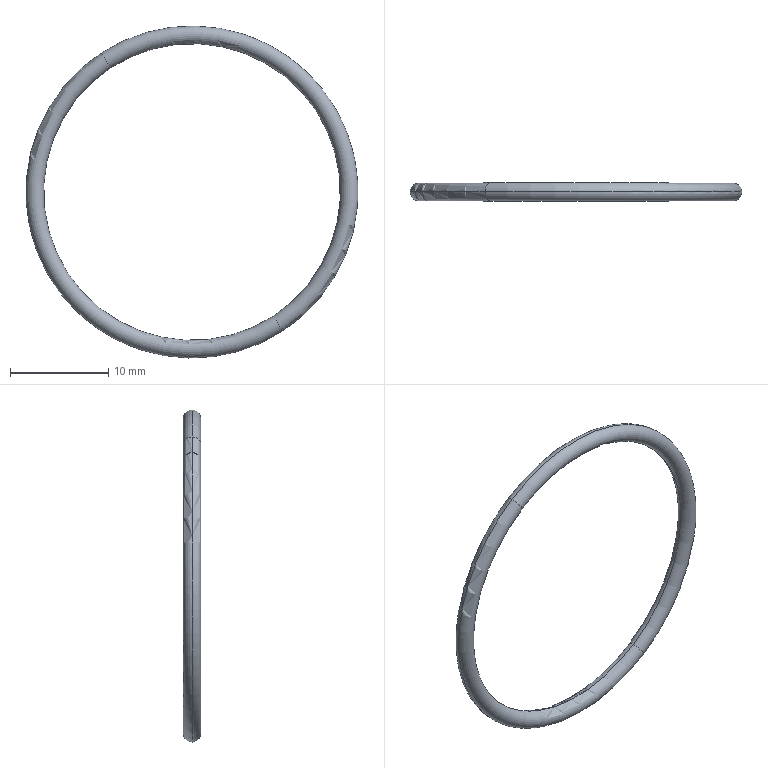Part | SolidWorks | features BaseBody 1 | 1 solid | 4 faces | box 33.8 x 1.8 x 33.8 mm | volume 255.82 mm3 | torus 4
STEP:
#1=CARTESIAN_POINT('',(218.757,-105.5,303.648));
#2=VERTEX_POINT('',#1);
#3=CARTESIAN_POINT('',(219.741,-105.5,302.141));
#4=VERTEX_POINT('',#3);
#5=CARTESIAN_POINT('',(219.249,-105.5,302.895));
#6=DIRECTION('',(-0.8372,0.,-0.5469));
#7=DIRECTION('',(-0.5469,0.,0.8372));
#8=AXIS2_PLACEMENT_3D('',#5,#6,#7);
#9=CIRCLE('',#8,0.9);
#10=EDGE_CURVE('',#2,#4,#9,.T.);
#11=ORIENTED_EDGE('',*,*,#10,.F.);
#12=CARTESIAN_POINT('',(237.243,-105.5,275.352));
#13=VERTEX_POINT('',#12);
#14=CARTESIAN_POINT('',(228.,-105.5,289.5));
#15=DIRECTION('',(0.,1.,0.));
#16=DIRECTION('',(0.,0.,1.));
#17=AXIS2_PLACEMENT_3D('',#14,#15,#16);
#18=CIRCLE('',#17,16.9);
#19=EDGE_CURVE('',#2,#13,#18,.T.);
#20=ORIENTED_EDGE('',*,*,#19,.T.);
#21=CARTESIAN_POINT('',(236.259,-105.5,276.859));
#22=VERTEX_POINT('',#21);
#23=CARTESIAN_POINT('',(236.751,-105.5,276.105));
#24=DIRECTION('',(0.8372,0.,0.5469));
#25=DIRECTION('',(0.5469,0.,-0.8372));
#26=AXIS2_PLACEMENT_3D('',#23,#24,#25);
#27=CIRCLE('',#26,0.9);
#28=EDGE_CURVE('',#13,#22,#27,.T.);
#29=ORIENTED_EDGE('',*,*,#28,.T.);
#30=CARTESIAN_POINT('',(228.,-105.5,289.5));
#31=DIRECTION('',(0.,1.,0.));
#32=DIRECTION('',(0.,0.,1.));
#33=AXIS2_PLACEMENT_3D('',#30,#31,#32);
#34=CIRCLE('',#33,15.1);
#35=EDGE_CURVE('',#4,#22,#34,.T.);
#36=ORIENTED_EDGE('',*,*,#35,.F.);
#37=EDGE_LOOP('',(#11,#20,#29,#36));
#38=FACE_OUTER_BOUND('',#37,.T.);
#39=CARTESIAN_POINT('',(228.,-105.5,289.5));
#40=DIRECTION('',(0.,1.,0.));
#41=DIRECTION('',(0.5469,0.,-0.8372));
#42=AXIS2_PLACEMENT_3D('',#39,#40,#41);
#43=TOROIDAL_SURFACE('',#42,16.,0.9);
#44=ADVANCED_FACE('',(#38),#43,.T.);
#45=ORIENTED_EDGE('',*,*,#28,.F.);
#46=CARTESIAN_POINT('',(228.,-105.5,289.5));
#47=DIRECTION('',(0.,1.,0.));
#48=DIRECTION('',(0.,0.,1.));
#49=AXIS2_PLACEMENT_3D('',#46,#47,#48);
#50=CIRCLE('',#49,16.9);
#51=EDGE_CURVE('',#13,#2,#50,.T.);
#52=ORIENTED_EDGE('',*,*,#51,.T.);
#53=ORIENTED_EDGE('',*,*,#10,.T.);
#54=CARTESIAN_POINT('',(228.,-105.5,289.5));
#55=DIRECTION('',(0.,1.,0.));
#56=DIRECTION('',(0.,0.,1.));
#57=AXIS2_PLACEMENT_3D('',#54,#55,#56);
#58=CIRCLE('',#57,15.1);
#59=EDGE_CURVE('',#22,#4,#58,.T.);
#60=ORIENTED_EDGE('',*,*,#59,.F.);
#61=EDGE_LOOP('',(#45,#52,#53,#60));
#62=FACE_OUTER_BOUND('',#61,.T.);
#63=CARTESIAN_POINT('',(228.,-105.5,289.5));
#64=DIRECTION('',(0.,1.,0.));
#65=DIRECTION('',(0.5469,0.,-0.8372));
#66=AXIS2_PLACEMENT_3D('',#63,#64,#65);
#67=TOROIDAL_SURFACE('',#66,16.,0.9);
#68=ADVANCED_FACE('',(#62),#67,.T.);
#69=ORIENTED_EDGE('',*,*,#51,.F.);
#70=CARTESIAN_POINT('',(236.751,-105.5,276.105));
#71=DIRECTION('',(0.8372,0.,0.5469));
#72=DIRECTION('',(0.5469,0.,-0.8372));
#73=AXIS2_PLACEMENT_3D('',#70,#71,#72);
#74=CIRCLE('',#73,0.9);
#75=EDGE_CURVE('',#22,#13,#74,.T.);
#76=ORIENTED_EDGE('',*,*,#75,.F.);
#77=ORIENTED_EDGE('',*,*,#59,.T.);
#78=CARTESIAN_POINT('',(219.249,-105.5,302.895));
#79=DIRECTION('',(-0.8372,0.,-0.5469));
#80=DIRECTION('',(-0.5469,0.,0.8372));
#81=AXIS2_PLACEMENT_3D('',#78,#79,#80);
#82=CIRCLE('',#81,0.9);
#83=EDGE_CURVE('',#4,#2,#82,.T.);
#84=ORIENTED_EDGE('',*,*,#83,.T.);
#85=EDGE_LOOP('',(#69,#76,#77,#84));
#86=FACE_OUTER_BOUND('',#85,.T.);
#87=CARTESIAN_POINT('',(228.,-105.5,289.5));
#88=DIRECTION('',(0.,1.,0.));
#89=DIRECTION('',(0.5469,0.,-0.8372));
#90=AXIS2_PLACEMENT_3D('',#87,#88,#89);
#91=TOROIDAL_SURFACE('',#90,16.,0.9);
#92=ADVANCED_FACE('',(#86),#91,.T.);
#93=ORIENTED_EDGE('',*,*,#19,.F.);
#94=ORIENTED_EDGE('',*,*,#83,.F.);
#95=ORIENTED_EDGE('',*,*,#35,.T.);
#96=ORIENTED_EDGE('',*,*,#75,.T.);
#97=EDGE_LOOP('',(#93,#94,#95,#96));
#98=FACE_OUTER_BOUND('',#97,.T.);
#99=CARTESIAN_POINT('',(228.,-105.5,289.5));
#100=DIRECTION('',(0.,1.,0.));
#101=DIRECTION('',(0.5469,0.,-0.8372));
#102=AXIS2_PLACEMENT_3D('',#99,#100,#101);
#103=TOROIDAL_SURFACE('',#102,16.,0.9);
#104=ADVANCED_FACE('',(#98),#103,.T.);
#105=CLOSED_SHELL('',(#44,#68,#92,#104));
#106=MANIFOLD_SOLID_BREP('',#105);
#107=CARTESIAN_POINT('',(0.,0.,0.));
#108=DIRECTION('',(0.,0.,1.));
#109=DIRECTION('',(1.,0.,0.));
#110=AXIS2_PLACEMENT_3D('',#107,#108,#109);
#111=(LENGTH_UNIT()NAMED_UNIT(*)SI_UNIT(.MILLI.,.METRE.));
#112=UNCERTAINTY_MEASURE_WITH_UNIT(LENGTH_MEASURE(0.00001),#111,'','');
#113=(NAMED_UNIT(*)PLANE_ANGLE_UNIT()SI_UNIT($,.RADIAN.));
#114=(NAMED_UNIT(*)SI_UNIT($,.STERADIAN.)SOLID_ANGLE_UNIT());
#115=(GEOMETRIC_REPRESENTATION_CONTEXT(3)GLOBAL_UNCERTAINTY_ASSIGNED_CONTEXT((#112))GLOBAL_UNIT_ASSIGNED_CONTEXT((#111,#113,#114))REPRESENTATION_CONTEXT('',''));
#116=ADVANCED_BREP_SHAPE_REPRESENTATION('',(#106,#110),#115);